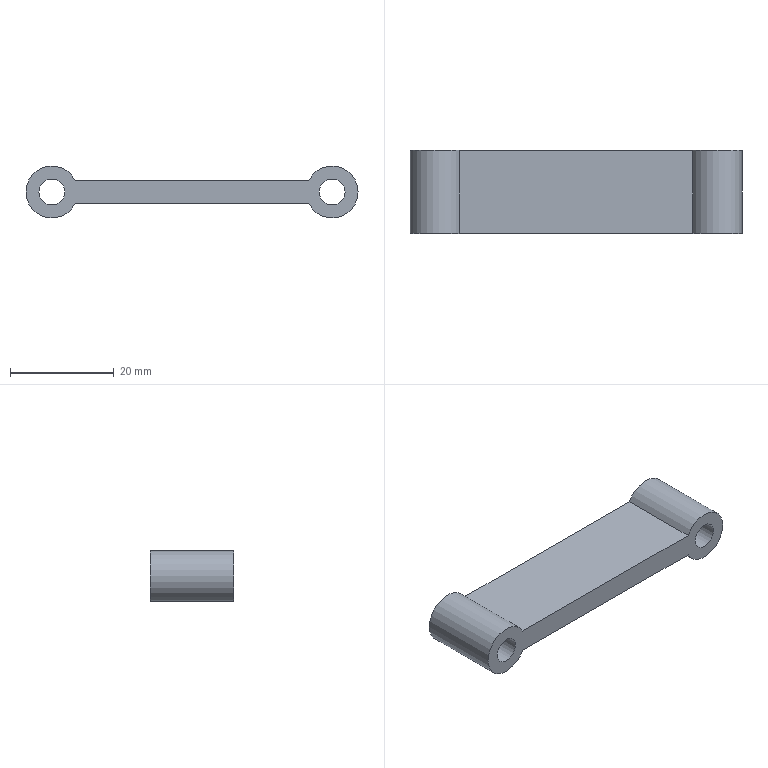Part | NX | features DATUM_CSYS 5, EXTRUDE 4, SKETCH 4 | 1 solid | 8 faces | box 64 x 16 x 10 mm | volume 5121 mm3 | cylinder 4 | plane 4 | commonest cylinder face diameters 5 x2 10 x2
STEP:
#1=CARTESIAN_POINT('',(4.45,0.,2.28));
#2=VERTEX_POINT('',#1);
#3=CARTESIAN_POINT('',(4.45,0.,-2.28));
#4=VERTEX_POINT('',#3);
#5=CARTESIAN_POINT('',(0.,0.,0.));
#6=DIRECTION('',(0.,-1.,0.));
#7=DIRECTION('',(1.,0.,0.));
#8=AXIS2_PLACEMENT_3D('',#5,#6,#7);
#9=CIRCLE('',#8,5.);
#10=EDGE_CURVE('',#2,#4,#9,.T.);
#11=ORIENTED_EDGE('',*,*,#10,.T.);
#12=CARTESIAN_POINT('',(4.45,-16.,-2.28));
#13=VERTEX_POINT('',#12);
#14=CARTESIAN_POINT('',(4.45,-16.,-2.28));
#15=DIRECTION('',(0.,1.,0.));
#16=VECTOR('',#15,1000.);
#17=LINE('',#14,#16);
#18=EDGE_CURVE('',#4,#13,#17,.F.);
#19=ORIENTED_EDGE('',*,*,#18,.T.);
#20=CARTESIAN_POINT('',(4.45,-16.,2.28));
#21=VERTEX_POINT('',#20);
#22=CARTESIAN_POINT('',(0.,-16.,0.));
#23=DIRECTION('',(0.,-1.,0.));
#24=DIRECTION('',(1.,0.,0.));
#25=AXIS2_PLACEMENT_3D('',#22,#23,#24);
#26=CIRCLE('',#25,5.);
#27=EDGE_CURVE('',#21,#13,#26,.T.);
#28=ORIENTED_EDGE('',*,*,#27,.F.);
#29=CARTESIAN_POINT('',(4.45,-16.,2.28));
#30=DIRECTION('',(0.,1.,0.));
#31=VECTOR('',#30,1000.);
#32=LINE('',#29,#31);
#33=EDGE_CURVE('',#21,#2,#32,.T.);
#34=ORIENTED_EDGE('',*,*,#33,.T.);
#35=EDGE_LOOP('',(#11,#19,#28,#34));
#36=FACE_BOUND('',#35,.T.);
#37=CARTESIAN_POINT('',(0.,-16.,0.));
#38=DIRECTION('',(0.,1.,0.));
#39=DIRECTION('',(0.,0.,1.));
#40=AXIS2_PLACEMENT_3D('',#37,#38,#39);
#41=CYLINDRICAL_SURFACE('',#40,5.);
#42=ADVANCED_FACE('',(#36),#41,.T.);
#43=CARTESIAN_POINT('',(2.5,-16.,0.));
#44=VERTEX_POINT('',#43);
#45=CARTESIAN_POINT('',(0.,-16.,0.));
#46=DIRECTION('',(0.,-1.,0.));
#47=DIRECTION('',(1.,0.,0.));
#48=AXIS2_PLACEMENT_3D('',#45,#46,#47);
#49=CIRCLE('',#48,2.5);
#50=EDGE_CURVE('',#44,#44,#49,.T.);
#51=ORIENTED_EDGE('',*,*,#50,.T.);
#52=EDGE_LOOP('',(#51));
#53=FACE_BOUND('',#52,.T.);
#54=CARTESIAN_POINT('',(2.5,0.,0.));
#55=VERTEX_POINT('',#54);
#56=CARTESIAN_POINT('',(0.,0.,0.));
#57=DIRECTION('',(0.,-1.,0.));
#58=DIRECTION('',(1.,0.,0.));
#59=AXIS2_PLACEMENT_3D('',#56,#57,#58);
#60=CIRCLE('',#59,2.5);
#61=EDGE_CURVE('',#55,#55,#60,.T.);
#62=ORIENTED_EDGE('',*,*,#61,.F.);
#63=EDGE_LOOP('',(#62));
#64=FACE_BOUND('',#63,.T.);
#65=CARTESIAN_POINT('',(0.,-16.,0.));
#66=DIRECTION('',(0.,1.,0.));
#67=DIRECTION('',(0.,0.,1.));
#68=AXIS2_PLACEMENT_3D('',#65,#66,#67);
#69=CYLINDRICAL_SURFACE('',#68,2.5);
#70=ADVANCED_FACE('',(#53,#64),#69,.F.);
#71=CARTESIAN_POINT('',(56.5,-16.,0.));
#72=VERTEX_POINT('',#71);
#73=CARTESIAN_POINT('',(54.,-16.,0.));
#74=DIRECTION('',(0.,-1.,0.));
#75=DIRECTION('',(1.,0.,0.));
#76=AXIS2_PLACEMENT_3D('',#73,#74,#75);
#77=CIRCLE('',#76,2.5);
#78=EDGE_CURVE('',#72,#72,#77,.T.);
#79=ORIENTED_EDGE('',*,*,#78,.F.);
#80=EDGE_LOOP('',(#79));
#81=FACE_BOUND('',#80,.T.);
#82=CARTESIAN_POINT('',(49.55,-16.,-2.28));
#83=VERTEX_POINT('',#82);
#84=CARTESIAN_POINT('',(49.55,-16.,2.28));
#85=VERTEX_POINT('',#84);
#86=CARTESIAN_POINT('',(54.,-16.,0.));
#87=DIRECTION('',(0.,-1.,0.));
#88=DIRECTION('',(1.,0.,0.));
#89=AXIS2_PLACEMENT_3D('',#86,#87,#88);
#90=CIRCLE('',#89,5.);
#91=EDGE_CURVE('',#83,#85,#90,.T.);
#92=ORIENTED_EDGE('',*,*,#91,.T.);
#93=CARTESIAN_POINT('',(54.,-16.,2.28));
#94=DIRECTION('',(-1.,0.,0.));
#95=VECTOR('',#94,1000.);
#96=LINE('',#93,#95);
#97=EDGE_CURVE('',#85,#21,#96,.T.);
#98=ORIENTED_EDGE('',*,*,#97,.T.);
#99=ORIENTED_EDGE('',*,*,#27,.T.);
#100=CARTESIAN_POINT('',(4.,-16.,-2.28));
#101=DIRECTION('',(1.,0.,0.));
#102=VECTOR('',#101,1000.);
#103=LINE('',#100,#102);
#104=EDGE_CURVE('',#13,#83,#103,.T.);
#105=ORIENTED_EDGE('',*,*,#104,.T.);
#106=EDGE_LOOP('',(#92,#98,#99,#105));
#107=FACE_BOUND('',#106,.T.);
#108=ORIENTED_EDGE('',*,*,#50,.F.);
#109=EDGE_LOOP('',(#108));
#110=FACE_BOUND('',#109,.T.);
#111=CARTESIAN_POINT('',(0.,-16.,0.));
#112=DIRECTION('',(0.,-1.,0.));
#113=DIRECTION('',(0.,0.,-1.));
#114=AXIS2_PLACEMENT_3D('',#111,#112,#113);
#115=PLANE('',#114);
#116=ADVANCED_FACE('',(#81,#107,#110),#115,.T.);
#117=CARTESIAN_POINT('',(56.5,0.,0.));
#118=VERTEX_POINT('',#117);
#119=CARTESIAN_POINT('',(54.,0.,0.));
#120=DIRECTION('',(0.,-1.,0.));
#121=DIRECTION('',(1.,0.,0.));
#122=AXIS2_PLACEMENT_3D('',#119,#120,#121);
#123=CIRCLE('',#122,2.5);
#124=EDGE_CURVE('',#118,#118,#123,.T.);
#125=ORIENTED_EDGE('',*,*,#124,.T.);
#126=EDGE_LOOP('',(#125));
#127=FACE_BOUND('',#126,.T.);
#128=CARTESIAN_POINT('',(49.55,0.,2.28));
#129=VERTEX_POINT('',#128);
#130=CARTESIAN_POINT('',(54.,0.,2.28));
#131=DIRECTION('',(-1.,0.,0.));
#132=VECTOR('',#131,1000.);
#133=LINE('',#130,#132);
#134=EDGE_CURVE('',#129,#2,#133,.T.);
#135=ORIENTED_EDGE('',*,*,#134,.F.);
#136=CARTESIAN_POINT('',(49.55,0.,-2.28));
#137=VERTEX_POINT('',#136);
#138=CARTESIAN_POINT('',(54.,0.,0.));
#139=DIRECTION('',(0.,-1.,0.));
#140=DIRECTION('',(1.,0.,0.));
#141=AXIS2_PLACEMENT_3D('',#138,#139,#140);
#142=CIRCLE('',#141,5.);
#143=EDGE_CURVE('',#137,#129,#142,.T.);
#144=ORIENTED_EDGE('',*,*,#143,.F.);
#145=CARTESIAN_POINT('',(4.,0.,-2.28));
#146=DIRECTION('',(1.,0.,0.));
#147=VECTOR('',#146,1000.);
#148=LINE('',#145,#147);
#149=EDGE_CURVE('',#4,#137,#148,.T.);
#150=ORIENTED_EDGE('',*,*,#149,.F.);
#151=ORIENTED_EDGE('',*,*,#10,.F.);
#152=EDGE_LOOP('',(#135,#144,#150,#151));
#153=FACE_BOUND('',#152,.T.);
#154=ORIENTED_EDGE('',*,*,#61,.T.);
#155=EDGE_LOOP('',(#154));
#156=FACE_BOUND('',#155,.T.);
#157=CARTESIAN_POINT('',(0.,0.,0.));
#158=DIRECTION('',(0.,-1.,0.));
#159=DIRECTION('',(0.,0.,-1.));
#160=AXIS2_PLACEMENT_3D('',#157,#158,#159);
#161=PLANE('',#160);
#162=ADVANCED_FACE('',(#127,#153,#156),#161,.F.);
#163=CARTESIAN_POINT('',(49.55,0.,-2.28));
#164=DIRECTION('',(0.,-1.,0.));
#165=VECTOR('',#164,1000.);
#166=LINE('',#163,#165);
#167=EDGE_CURVE('',#83,#137,#166,.F.);
#168=ORIENTED_EDGE('',*,*,#167,.F.);
#169=ORIENTED_EDGE('',*,*,#104,.F.);
#170=ORIENTED_EDGE('',*,*,#18,.F.);
#171=ORIENTED_EDGE('',*,*,#149,.T.);
#172=EDGE_LOOP('',(#168,#169,#170,#171));
#173=FACE_BOUND('',#172,.T.);
#174=CARTESIAN_POINT('',(4.,0.,-2.28));
#175=DIRECTION('',(0.,0.,-1.));
#176=DIRECTION('',(-1.,0.,0.));
#177=AXIS2_PLACEMENT_3D('',#174,#175,#176);
#178=PLANE('',#177);
#179=ADVANCED_FACE('',(#173),#178,.T.);
#180=CARTESIAN_POINT('',(49.55,0.,2.28));
#181=DIRECTION('',(0.,-1.,0.));
#182=VECTOR('',#181,1000.);
#183=LINE('',#180,#182);
#184=EDGE_CURVE('',#129,#85,#183,.T.);
#185=ORIENTED_EDGE('',*,*,#184,.F.);
#186=ORIENTED_EDGE('',*,*,#134,.T.);
#187=ORIENTED_EDGE('',*,*,#33,.F.);
#188=ORIENTED_EDGE('',*,*,#97,.F.);
#189=EDGE_LOOP('',(#185,#186,#187,#188));
#190=FACE_BOUND('',#189,.T.);
#191=CARTESIAN_POINT('',(54.,0.,2.28));
#192=DIRECTION('',(0.,0.,1.));
#193=DIRECTION('',(1.,0.,0.));
#194=AXIS2_PLACEMENT_3D('',#191,#192,#193);
#195=PLANE('',#194);
#196=ADVANCED_FACE('',(#190),#195,.T.);
#197=ORIENTED_EDGE('',*,*,#91,.F.);
#198=ORIENTED_EDGE('',*,*,#167,.T.);
#199=ORIENTED_EDGE('',*,*,#143,.T.);
#200=ORIENTED_EDGE('',*,*,#184,.T.);
#201=EDGE_LOOP('',(#197,#198,#199,#200));
#202=FACE_BOUND('',#201,.T.);
#203=CARTESIAN_POINT('',(54.,0.,0.));
#204=DIRECTION('',(0.,-1.,0.));
#205=DIRECTION('',(0.,0.,-1.));
#206=AXIS2_PLACEMENT_3D('',#203,#204,#205);
#207=CYLINDRICAL_SURFACE('',#206,5.);
#208=ADVANCED_FACE('',(#202),#207,.T.);
#209=ORIENTED_EDGE('',*,*,#124,.F.);
#210=EDGE_LOOP('',(#209));
#211=FACE_BOUND('',#210,.T.);
#212=ORIENTED_EDGE('',*,*,#78,.T.);
#213=EDGE_LOOP('',(#212));
#214=FACE_BOUND('',#213,.T.);
#215=CARTESIAN_POINT('',(54.,0.,0.));
#216=DIRECTION('',(0.,-1.,0.));
#217=DIRECTION('',(0.,0.,-1.));
#218=AXIS2_PLACEMENT_3D('',#215,#216,#217);
#219=CYLINDRICAL_SURFACE('',#218,2.5);
#220=ADVANCED_FACE('',(#211,#214),#219,.F.);
#221=CLOSED_SHELL('',(#42,#70,#116,#162,#179,#196,#208,#220));
#222=MANIFOLD_SOLID_BREP('',#221);
#223=(LENGTH_UNIT()NAMED_UNIT(*)SI_UNIT(.MILLI.,.METRE.));
#224=UNCERTAINTY_MEASURE_WITH_UNIT(LENGTH_MEASURE(0.00001),#223,'','');
#225=(NAMED_UNIT(*)PLANE_ANGLE_UNIT()SI_UNIT($,.RADIAN.));
#226=(NAMED_UNIT(*)SI_UNIT($,.STERADIAN.)SOLID_ANGLE_UNIT());
#227=(GEOMETRIC_REPRESENTATION_CONTEXT(3)GLOBAL_UNCERTAINTY_ASSIGNED_CONTEXT((#224))GLOBAL_UNIT_ASSIGNED_CONTEXT((#223,#225,#226))REPRESENTATION_CONTEXT('',''));
#228=ADVANCED_BREP_SHAPE_REPRESENTATION('',(#222),#227);